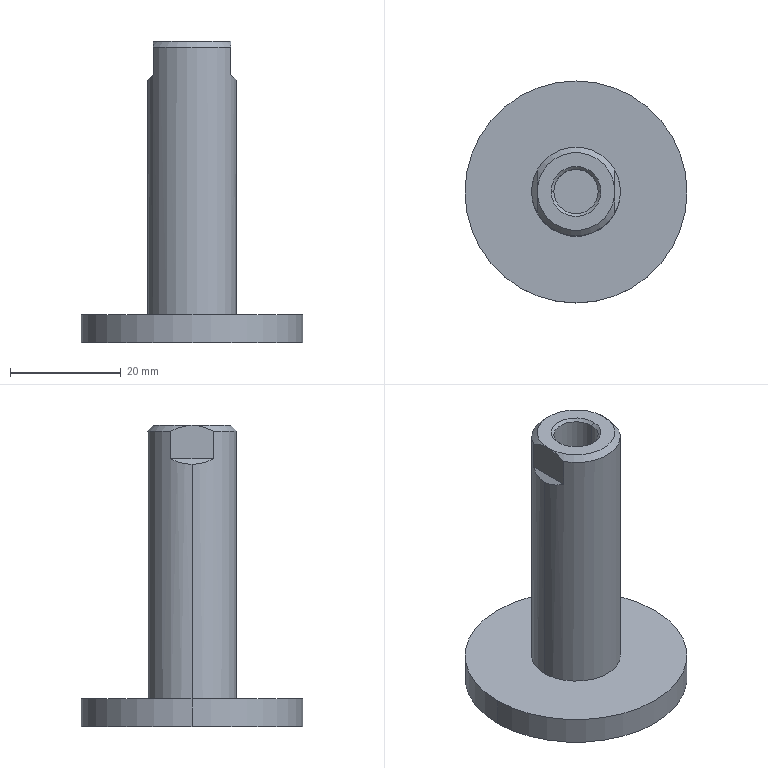Part | STEP file | CQ2B40-30D_CQ22031Rods | 1 solid | 18 faces | box 40 x 40 x 54.25 mm | volume 15444 mm3 | plane 8 | cylinder 6 | cone 4 | commonest cylinder face diameters 8 x2 16 x2 40 x2